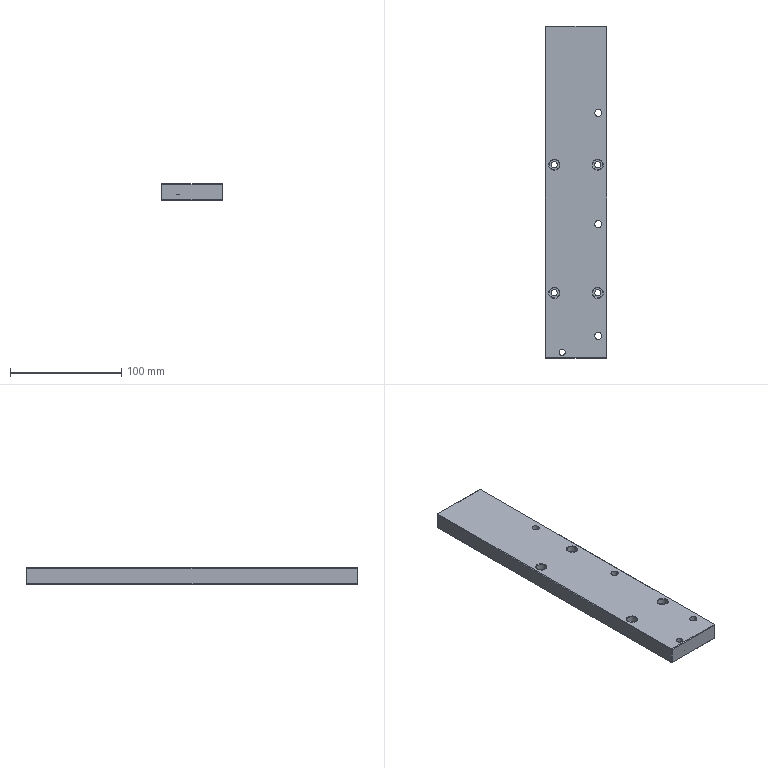CAM job | NX | 3-axis milling, drilling | part box 55 x 298 x 15 mm | stock box 55 x 298 x 15 mm
Tools:
number,name,description,diameter,corner_radius,flute_length,length,flutes
4,D4,平底铣刀-粗,4.0,0.0,25.0,75.0,2
6,D6,平底铣刀-粗,6.0,0.0,25.0,75.0,2
11,D4-J,平底铣刀-精,4.0,0.0,50.0,75.0,2
7,D6-J,平底铣刀-精,6.0,0.0,25.0,75.0,2
2,D6倒角刀,倒角刀,6.0,0.0,3.0,25.0,2
1,C6定点钻,倒角刀,6.0,0.0,3.0,3.0,2
18,ZT6.5,钻头,6.5,0.0,35.0,50.0,2
17,钻头5.5,Twist Drill 5 mm,5.5,0.0,52.0,54.0,2
Operations:
program,operation,operation_type,tool,method,geometry_group,spindle_rpm,surface_speed,feed_per_tooth,feed_cut,feed_plunge,cut_length_mm,path_length_mm,cut_time_min,machine_time_min
B,孔粗_1,CylinderMilling,D6,METHOD,W-B,3000.0,56.549,0.1667,1000.0,100.0,290.386,335.086,0.2904,0.2949
B,孔粗_2,CylinderMilling,D6,METHOD,W-B,3000.0,56.549,0.1667,1000.0,100.0,728.708,1165.808,0.7287,0.7724
B,铣倒角_4,PlanarMilling,D6倒角刀,METHOD,W-B,4000.0,75.398,0.075,600.0,100.0,51.33,413.958,0.0855,0.1218
B,铣倒角_5,PlanarMilling,D6倒角刀,METHOD,W-B,3000.0,56.549,0.1,600.0,100.0,23.42,67.42,0.039,0.0434
B,铣倒角_6,PlanarMilling,D6倒角刀,METHOD,W-B,3000.0,56.549,0.1,600.0,100.0,100.496,442.36,0.1675,0.2017
B,底壁铣倒角_COPY,VolumeBased25DMillingOperation,D6倒角刀,爬面_倒角-切深0-步距G,W-B,3500.0,65.972,0.1429,1000.0,100.0,718.77,758.17,0.7188,0.7227
B,孔侧_1,CylinderMilling,D6-J,METHOD,W-B,3500.0,65.973,0.0857,600.0,100.0,13.425,64.425,0.0224,0.0275
B,孔侧_2,CylinderMilling,D6-J,METHOD,W-B,3500.0,65.973,0.1143,800.0,100.0,65.075,524.075,0.0813,0.1272
A,打点-深0.8,Operation,C6定点钻,NONE,W-A,3000.0,56.0,0.01,60.0,90.0,14.4,414.272,0.24,0.28
A,通孔-5-6,Operation,钻头5.5,NONE,W-A,1000.0,17.279,0.04,80.0,90.0,19.0,78.0,0.2375,0.2434
A,沉头孔-钻孔0段,Operation,钻头5.5,NONE,W-A,1000.0,17.279,0.04,80.0,90.0,78.609,393.249,0.9826,1.014
A,通孔-6-8,Operation,ZT6.5,NONE,W-A,800.0,16.336,0.0625,100.0,90.0,57.0,356.01,0.57,0.5999
A,铣孔开粗D4_1,CylinderMilling,D4,NONE,W-A,4000.0,50.266,0.25,2000.0,100.0,3076.773,3473.773,1.538,1.578
A,铣孔精光D4_1,CylinderMilling,D4-J,精光步距切深关,W-A,4000.0,50.266,0.1,800.0,100.0,179.78,550.78,0.2247,0.2618
A,铣倒角_1,PlanarMilling,D6倒角刀,METHOD,W-A,4000.0,75.398,0.0375,300.0,100.0,20.704,61.304,0.069,0.0731
A,铣倒角_2,PlanarMilling,D6倒角刀,METHOD,W-A,4000.0,75.398,0.05,400.0,100.0,69.16,386.161,0.1729,0.2046
A,铣倒角_3,PlanarMilling,D6倒角刀,NONE,W-A,4000.0,75.398,0.0625,500.0,100.0,146.746,485.457,0.2935,0.3274
A,C0.3封闭铣廓倒角6X45L_COPY,PlanarMilling,D6倒角刀,爬面_倒角-切深0-步距G,W-A,4000.0,75.398,0.125,1000.0,100.0,726.12,762.62,0.7261,0.7298